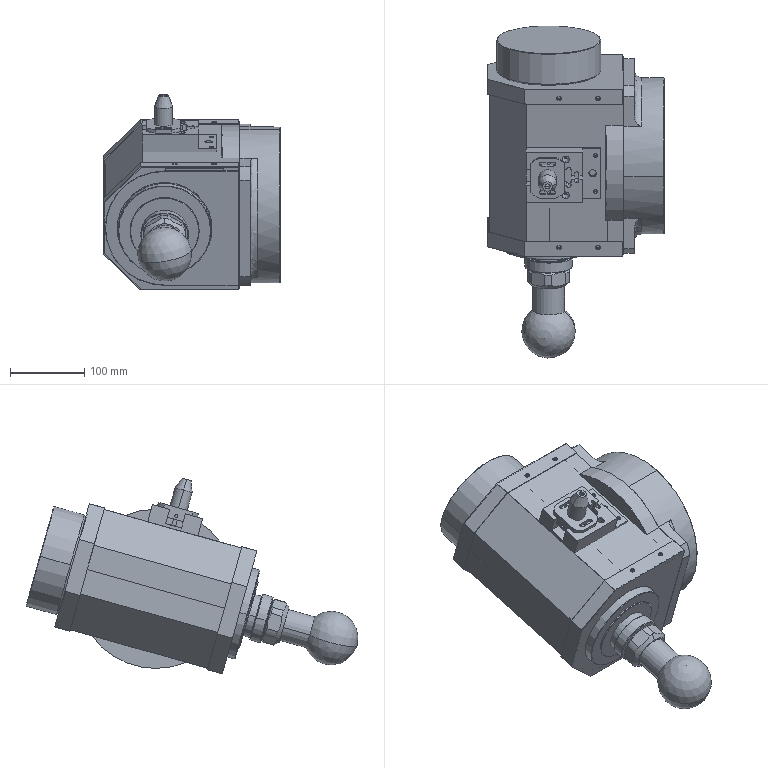Part | SolidWorks | 13 solids | 669 faces | box 237.6 x 446.584 x 263.499 mm | volume 8299618 mm3 | cylinder 265 | plane 245 | cone 155 | spline 2 | sphere 2 | commonest cylinder face diameters 5 x42 9 x24 5.5 x17 6.5 x16 14.5 x16 6 x11